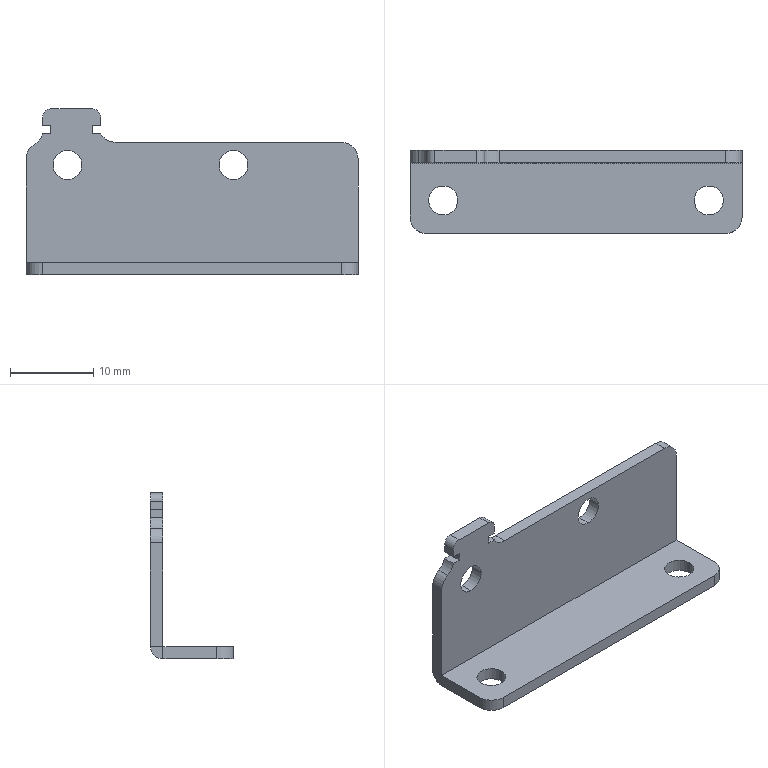Part | SolidWorks | features Fillet 3, ICE 3, FlatPattern 1, SMBaseFlange 1, SheetMetal 1 | 1 solid | 38 faces | box 40 x 10 x 20 mm | volume 1427 mm3 | plane 21 | cylinder 17 | commonest cylinder face diameters 3.5 x8 4 x6 2 x2 3 x1
STEP:
#1=CARTESIAN_POINT('',(5.75,-6.,-16.));
#2=VERTEX_POINT('',#1);
#3=CARTESIAN_POINT('',(2.25,-6.,-16.));
#4=VERTEX_POINT('',#3);
#5=CARTESIAN_POINT('',(4.,-6.,-16.));
#6=DIRECTION('',(0.,0.,-1.));
#7=DIRECTION('',(0.,1.,0.));
#8=AXIS2_PLACEMENT_3D('',#5,#6,#7);
#9=CIRCLE('',#8,1.75);
#10=EDGE_CURVE('',#2,#4,#9,.T.);
#11=ORIENTED_EDGE('',*,*,#10,.T.);
#12=CARTESIAN_POINT('',(2.25,-6.,-14.5));
#13=VERTEX_POINT('',#12);
#14=CARTESIAN_POINT('',(2.25,-6.,-24.5));
#15=DIRECTION('',(0.,0.,1.));
#16=VECTOR('',#15,1000.);
#17=LINE('',#14,#16);
#18=EDGE_CURVE('',#4,#13,#17,.T.);
#19=ORIENTED_EDGE('',*,*,#18,.T.);
#20=CARTESIAN_POINT('',(5.75,-6.,-14.5));
#21=VERTEX_POINT('',#20);
#22=CARTESIAN_POINT('',(4.,-6.,-14.5));
#23=DIRECTION('',(0.,0.,1.));
#24=DIRECTION('',(1.,0.,0.));
#25=AXIS2_PLACEMENT_3D('',#22,#23,#24);
#26=CIRCLE('',#25,1.75);
#27=EDGE_CURVE('',#13,#21,#26,.T.);
#28=ORIENTED_EDGE('',*,*,#27,.T.);
#29=CARTESIAN_POINT('',(5.75,-6.,-24.5));
#30=DIRECTION('',(0.,0.,1.));
#31=VECTOR('',#30,1000.);
#32=LINE('',#29,#31);
#33=EDGE_CURVE('',#2,#21,#32,.T.);
#34=ORIENTED_EDGE('',*,*,#33,.F.);
#35=EDGE_LOOP('',(#11,#19,#28,#34));
#36=FACE_OUTER_BOUND('',#35,.T.);
#37=CARTESIAN_POINT('',(4.,-6.,-24.5));
#38=DIRECTION('',(0.,0.,1.));
#39=DIRECTION('',(1.,0.,0.));
#40=AXIS2_PLACEMENT_3D('',#37,#38,#39);
#41=CYLINDRICAL_SURFACE('',#40,1.75);
#42=ADVANCED_FACE('',(#36),#41,.F.);
#43=CARTESIAN_POINT('',(37.75,-6.,-16.));
#44=VERTEX_POINT('',#43);
#45=CARTESIAN_POINT('',(34.25,-6.,-16.));
#46=VERTEX_POINT('',#45);
#47=CARTESIAN_POINT('',(36.,-6.,-16.));
#48=DIRECTION('',(0.,0.,-1.));
#49=DIRECTION('',(0.,1.,0.));
#50=AXIS2_PLACEMENT_3D('',#47,#48,#49);
#51=CIRCLE('',#50,1.75);
#52=EDGE_CURVE('',#44,#46,#51,.T.);
#53=ORIENTED_EDGE('',*,*,#52,.T.);
#54=CARTESIAN_POINT('',(34.25,-6.,-14.5));
#55=VERTEX_POINT('',#54);
#56=CARTESIAN_POINT('',(34.25,-6.,-24.5));
#57=DIRECTION('',(0.,0.,1.));
#58=VECTOR('',#57,1000.);
#59=LINE('',#56,#58);
#60=EDGE_CURVE('',#46,#55,#59,.T.);
#61=ORIENTED_EDGE('',*,*,#60,.T.);
#62=CARTESIAN_POINT('',(37.75,-6.,-14.5));
#63=VERTEX_POINT('',#62);
#64=CARTESIAN_POINT('',(36.,-6.,-14.5));
#65=DIRECTION('',(0.,0.,1.));
#66=DIRECTION('',(1.,0.,0.));
#67=AXIS2_PLACEMENT_3D('',#64,#65,#66);
#68=CIRCLE('',#67,1.75);
#69=EDGE_CURVE('',#55,#63,#68,.T.);
#70=ORIENTED_EDGE('',*,*,#69,.T.);
#71=CARTESIAN_POINT('',(37.75,-6.,-24.5));
#72=DIRECTION('',(0.,0.,1.));
#73=VECTOR('',#72,1000.);
#74=LINE('',#71,#73);
#75=EDGE_CURVE('',#44,#63,#74,.T.);
#76=ORIENTED_EDGE('',*,*,#75,.F.);
#77=EDGE_LOOP('',(#53,#61,#70,#76));
#78=FACE_OUTER_BOUND('',#77,.T.);
#79=CARTESIAN_POINT('',(36.,-6.,-24.5));
#80=DIRECTION('',(0.,0.,1.));
#81=DIRECTION('',(1.,0.,0.));
#82=AXIS2_PLACEMENT_3D('',#79,#80,#81);
#83=CYLINDRICAL_SURFACE('',#82,1.75);
#84=ADVANCED_FACE('',(#78),#83,.F.);
#85=CARTESIAN_POINT('',(5.,0.,-4.5));
#86=VERTEX_POINT('',#85);
#87=CARTESIAN_POINT('',(5.,0.,-1.));
#88=VERTEX_POINT('',#87);
#89=CARTESIAN_POINT('',(5.,0.,-2.75));
#90=DIRECTION('',(0.,1.,0.));
#91=DIRECTION('',(0.,0.,1.));
#92=AXIS2_PLACEMENT_3D('',#89,#90,#91);
#93=CIRCLE('',#92,1.75);
#94=EDGE_CURVE('',#86,#88,#93,.T.);
#95=ORIENTED_EDGE('',*,*,#94,.T.);
#96=CARTESIAN_POINT('',(5.,-1.5,-1.));
#97=VERTEX_POINT('',#96);
#98=CARTESIAN_POINT('',(5.,8.5,-1.));
#99=DIRECTION('',(0.,-1.,0.));
#100=VECTOR('',#99,1000.);
#101=LINE('',#98,#100);
#102=EDGE_CURVE('',#88,#97,#101,.T.);
#103=ORIENTED_EDGE('',*,*,#102,.T.);
#104=CARTESIAN_POINT('',(5.,-1.5,-4.5));
#105=VERTEX_POINT('',#104);
#106=CARTESIAN_POINT('',(5.,-1.5,-2.75));
#107=DIRECTION('',(0.,-1.,0.));
#108=DIRECTION('',(0.,0.,-1.));
#109=AXIS2_PLACEMENT_3D('',#106,#107,#108);
#110=CIRCLE('',#109,1.75);
#111=EDGE_CURVE('',#97,#105,#110,.T.);
#112=ORIENTED_EDGE('',*,*,#111,.T.);
#113=CARTESIAN_POINT('',(5.,8.5,-4.5));
#114=DIRECTION('',(0.,-1.,0.));
#115=VECTOR('',#114,1000.);
#116=LINE('',#113,#115);
#117=EDGE_CURVE('',#86,#105,#116,.T.);
#118=ORIENTED_EDGE('',*,*,#117,.F.);
#119=EDGE_LOOP('',(#95,#103,#112,#118));
#120=FACE_OUTER_BOUND('',#119,.T.);
#121=CARTESIAN_POINT('',(5.,8.5,-2.75));
#122=DIRECTION('',(0.,-1.,0.));
#123=DIRECTION('',(0.,0.,-1.));
#124=AXIS2_PLACEMENT_3D('',#121,#122,#123);
#125=CYLINDRICAL_SURFACE('',#124,1.75);
#126=ADVANCED_FACE('',(#120),#125,.F.);
#127=CARTESIAN_POINT('',(25.,0.,-4.5));
#128=VERTEX_POINT('',#127);
#129=CARTESIAN_POINT('',(25.,0.,-1.));
#130=VERTEX_POINT('',#129);
#131=CARTESIAN_POINT('',(25.,0.,-2.75));
#132=DIRECTION('',(0.,1.,0.));
#133=DIRECTION('',(0.,0.,1.));
#134=AXIS2_PLACEMENT_3D('',#131,#132,#133);
#135=CIRCLE('',#134,1.75);
#136=EDGE_CURVE('',#128,#130,#135,.T.);
#137=ORIENTED_EDGE('',*,*,#136,.T.);
#138=CARTESIAN_POINT('',(25.,-1.5,-1.));
#139=VERTEX_POINT('',#138);
#140=CARTESIAN_POINT('',(25.,8.5,-1.));
#141=DIRECTION('',(0.,-1.,0.));
#142=VECTOR('',#141,1000.);
#143=LINE('',#140,#142);
#144=EDGE_CURVE('',#130,#139,#143,.T.);
#145=ORIENTED_EDGE('',*,*,#144,.T.);
#146=CARTESIAN_POINT('',(25.,-1.5,-4.5));
#147=VERTEX_POINT('',#146);
#148=CARTESIAN_POINT('',(25.,-1.5,-2.75));
#149=DIRECTION('',(0.,-1.,0.));
#150=DIRECTION('',(0.,0.,-1.));
#151=AXIS2_PLACEMENT_3D('',#148,#149,#150);
#152=CIRCLE('',#151,1.75);
#153=EDGE_CURVE('',#139,#147,#152,.T.);
#154=ORIENTED_EDGE('',*,*,#153,.T.);
#155=CARTESIAN_POINT('',(25.,8.5,-4.5));
#156=DIRECTION('',(0.,-1.,0.));
#157=VECTOR('',#156,1000.);
#158=LINE('',#155,#157);
#159=EDGE_CURVE('',#128,#147,#158,.T.);
#160=ORIENTED_EDGE('',*,*,#159,.F.);
#161=EDGE_LOOP('',(#137,#145,#154,#160));
#162=FACE_OUTER_BOUND('',#161,.T.);
#163=CARTESIAN_POINT('',(25.,8.5,-2.75));
#164=DIRECTION('',(0.,-1.,0.));
#165=DIRECTION('',(0.,0.,-1.));
#166=AXIS2_PLACEMENT_3D('',#163,#164,#165);
#167=CYLINDRICAL_SURFACE('',#166,1.75);
#168=ADVANCED_FACE('',(#162),#167,.F.);
#169=CARTESIAN_POINT('',(40.,-1.5,-14.5));
#170=VERTEX_POINT('',#169);
#171=CARTESIAN_POINT('',(40.,-8.,-14.5));
#172=VERTEX_POINT('',#171);
#173=CARTESIAN_POINT('',(40.,0.,-14.5));
#174=DIRECTION('',(0.,-1.,0.));
#175=VECTOR('',#174,1000.);
#176=LINE('',#173,#175);
#177=EDGE_CURVE('',#170,#172,#176,.T.);
#178=ORIENTED_EDGE('',*,*,#177,.T.);
#179=CARTESIAN_POINT('',(40.,-8.,-16.));
#180=VERTEX_POINT('',#179);
#181=CARTESIAN_POINT('',(40.,-8.,-14.5));
#182=DIRECTION('',(0.,0.,-1.));
#183=VECTOR('',#182,1000.);
#184=LINE('',#181,#183);
#185=EDGE_CURVE('',#172,#180,#184,.T.);
#186=ORIENTED_EDGE('',*,*,#185,.T.);
#187=CARTESIAN_POINT('',(40.,-1.5,-16.));
#188=VERTEX_POINT('',#187);
#189=CARTESIAN_POINT('',(40.,0.,-16.));
#190=DIRECTION('',(0.,-1.,0.));
#191=VECTOR('',#190,1000.);
#192=LINE('',#189,#191);
#193=EDGE_CURVE('',#188,#180,#192,.T.);
#194=ORIENTED_EDGE('',*,*,#193,.F.);
#195=CARTESIAN_POINT('',(40.,-1.5,-14.5));
#196=DIRECTION('',(0.,0.,-1.));
#197=VECTOR('',#196,1000.);
#198=LINE('',#195,#197);
#199=EDGE_CURVE('',#170,#188,#198,.T.);
#200=ORIENTED_EDGE('',*,*,#199,.F.);
#201=EDGE_LOOP('',(#178,#186,#194,#200));
#202=FACE_OUTER_BOUND('',#201,.T.);
#203=CARTESIAN_POINT('',(40.,-1.5,-14.5));
#204=DIRECTION('',(1.,0.,0.));
#205=DIRECTION('',(0.,0.,-1.));
#206=AXIS2_PLACEMENT_3D('',#203,#204,#205);
#207=PLANE('',#206);
#208=ADVANCED_FACE('',(#202),#207,.T.);
#209=CARTESIAN_POINT('',(40.,0.,-14.5));
#210=VERTEX_POINT('',#209);
#211=CARTESIAN_POINT('',(40.,-1.5,-14.5));
#212=DIRECTION('',(0.,1.,0.));
#213=VECTOR('',#212,1000.);
#214=LINE('',#211,#213);
#215=EDGE_CURVE('',#170,#210,#214,.T.);
#216=ORIENTED_EDGE('',*,*,#215,.F.);
#217=ORIENTED_EDGE('',*,*,#199,.T.);
#218=CARTESIAN_POINT('',(40.,-1.5,-14.5));
#219=DIRECTION('',(-1.,0.,0.));
#220=DIRECTION('',(0.,0.,-1.));
#221=AXIS2_PLACEMENT_3D('',#218,#219,#220);
#222=CIRCLE('',#221,1.5);
#223=EDGE_CURVE('',#210,#188,#222,.T.);
#224=ORIENTED_EDGE('',*,*,#223,.F.);
#225=EDGE_LOOP('',(#216,#217,#224));
#226=FACE_OUTER_BOUND('',#225,.T.);
#227=CARTESIAN_POINT('',(40.,-1.5,-14.5));
#228=DIRECTION('',(1.,0.,0.));
#229=DIRECTION('',(0.,0.,-1.));
#230=AXIS2_PLACEMENT_3D('',#227,#228,#229);
#231=PLANE('',#230);
#232=ADVANCED_FACE('',(#226),#231,.T.);
#233=CARTESIAN_POINT('',(0.,-1.5,-2.));
#234=VERTEX_POINT('',#233);
#235=CARTESIAN_POINT('',(0.,-1.5,-14.5));
#236=VERTEX_POINT('',#235);
#237=CARTESIAN_POINT('',(0.,-1.5,0.));
#238=DIRECTION('',(0.,0.,-1.));
#239=VECTOR('',#238,1000.);
#240=LINE('',#237,#239);
#241=EDGE_CURVE('',#234,#236,#240,.T.);
#242=ORIENTED_EDGE('',*,*,#241,.F.);
#243=CARTESIAN_POINT('',(0.,0.,-2.));
#244=VERTEX_POINT('',#243);
#245=CARTESIAN_POINT('',(0.,-1.5,-2.));
#246=DIRECTION('',(0.,1.,0.));
#247=VECTOR('',#246,1000.);
#248=LINE('',#245,#247);
#249=EDGE_CURVE('',#234,#244,#248,.T.);
#250=ORIENTED_EDGE('',*,*,#249,.T.);
#251=CARTESIAN_POINT('',(0.,0.,-14.5));
#252=VERTEX_POINT('',#251);
#253=CARTESIAN_POINT('',(0.,0.,0.));
#254=DIRECTION('',(0.,0.,-1.));
#255=VECTOR('',#254,1000.);
#256=LINE('',#253,#255);
#257=EDGE_CURVE('',#244,#252,#256,.T.);
#258=ORIENTED_EDGE('',*,*,#257,.T.);
#259=CARTESIAN_POINT('',(0.,-1.5,-14.5));
#260=DIRECTION('',(0.,1.,0.));
#261=VECTOR('',#260,1000.);
#262=LINE('',#259,#261);
#263=EDGE_CURVE('',#236,#252,#262,.T.);
#264=ORIENTED_EDGE('',*,*,#263,.F.);
#265=EDGE_LOOP('',(#242,#250,#258,#264));
#266=FACE_OUTER_BOUND('',#265,.T.);
#267=CARTESIAN_POINT('',(0.,-1.5,-14.5));
#268=DIRECTION('',(-1.,0.,0.));
#269=DIRECTION('',(0.,0.,1.));
#270=AXIS2_PLACEMENT_3D('',#267,#268,#269);
#271=PLANE('',#270);
#272=ADVANCED_FACE('',(#266),#271,.T.);
#273=CARTESIAN_POINT('',(0.,-1.5,-16.));
#274=VERTEX_POINT('',#273);
#275=CARTESIAN_POINT('',(0.,-1.5,-14.5));
#276=DIRECTION('',(0.,0.,-1.));
#277=VECTOR('',#276,1000.);
#278=LINE('',#275,#277);
#279=EDGE_CURVE('',#236,#274,#278,.T.);
#280=ORIENTED_EDGE('',*,*,#279,.F.);
#281=ORIENTED_EDGE('',*,*,#263,.T.);
#282=CARTESIAN_POINT('',(0.,-1.5,-14.5));
#283=DIRECTION('',(-1.,0.,0.));
#284=DIRECTION('',(0.,0.,-1.));
#285=AXIS2_PLACEMENT_3D('',#282,#283,#284);
#286=CIRCLE('',#285,1.5);
#287=EDGE_CURVE('',#252,#274,#286,.T.);
#288=ORIENTED_EDGE('',*,*,#287,.T.);
#289=EDGE_LOOP('',(#280,#281,#288));
#290=FACE_OUTER_BOUND('',#289,.T.);
#291=CARTESIAN_POINT('',(0.,-1.5,-14.5));
#292=DIRECTION('',(-1.,0.,0.));
#293=DIRECTION('',(0.,0.,1.));
#294=AXIS2_PLACEMENT_3D('',#291,#292,#293);
#295=PLANE('',#294);
#296=ADVANCED_FACE('',(#290),#295,.T.);
#297=CARTESIAN_POINT('',(4.,-6.,-14.5));
#298=DIRECTION('',(0.,0.,1.));
#299=DIRECTION('',(1.,0.,0.));
#300=AXIS2_PLACEMENT_3D('',#297,#298,#299);
#301=CIRCLE('',#300,1.75);
#302=EDGE_CURVE('',#21,#13,#301,.T.);
#303=ORIENTED_EDGE('',*,*,#302,.F.);
#304=ORIENTED_EDGE('',*,*,#27,.F.);
#305=EDGE_LOOP('',(#303,#304));
#306=FACE_BOUND('',#305,.T.);
#307=CARTESIAN_POINT('',(36.,-6.,-14.5));
#308=DIRECTION('',(0.,0.,1.));
#309=DIRECTION('',(1.,0.,0.));
#310=AXIS2_PLACEMENT_3D('',#307,#308,#309);
#311=CIRCLE('',#310,1.75);
#312=EDGE_CURVE('',#63,#55,#311,.T.);
#313=ORIENTED_EDGE('',*,*,#312,.F.);
#314=ORIENTED_EDGE('',*,*,#69,.F.);
#315=EDGE_LOOP('',(#313,#314));
#316=FACE_BOUND('',#315,.T.);
#317=CARTESIAN_POINT('',(38.,-10.,-14.5));
#318=VERTEX_POINT('',#317);
#319=CARTESIAN_POINT('',(2.,-10.,-14.5));
#320=VERTEX_POINT('',#319);
#321=CARTESIAN_POINT('',(40.,-10.,-14.5));
#322=DIRECTION('',(-1.,0.,0.));
#323=VECTOR('',#322,1000.);
#324=LINE('',#321,#323);
#325=EDGE_CURVE('',#318,#320,#324,.T.);
#326=ORIENTED_EDGE('',*,*,#325,.F.);
#327=CARTESIAN_POINT('',(38.,-8.,-14.5));
#328=DIRECTION('',(0.,0.,1.));
#329=DIRECTION('',(0.,1.,0.));
#330=AXIS2_PLACEMENT_3D('',#327,#328,#329);
#331=CIRCLE('',#330,2.);
#332=EDGE_CURVE('',#318,#172,#331,.T.);
#333=ORIENTED_EDGE('',*,*,#332,.T.);
#334=ORIENTED_EDGE('',*,*,#177,.F.);
#335=CARTESIAN_POINT('',(40.,-1.5,-14.5));
#336=DIRECTION('',(-1.,0.,0.));
#337=VECTOR('',#336,1000.);
#338=LINE('',#335,#337);
#339=EDGE_CURVE('',#170,#236,#338,.T.);
#340=ORIENTED_EDGE('',*,*,#339,.T.);
#341=CARTESIAN_POINT('',(0.,-8.,-14.5));
#342=VERTEX_POINT('',#341);
#343=CARTESIAN_POINT('',(0.,0.,-14.5));
#344=DIRECTION('',(0.,-1.,0.));
#345=VECTOR('',#344,1000.);
#346=LINE('',#343,#345);
#347=EDGE_CURVE('',#236,#342,#346,.T.);
#348=ORIENTED_EDGE('',*,*,#347,.T.);
#349=CARTESIAN_POINT('',(2.,-8.,-14.5));
#350=DIRECTION('',(0.,0.,1.));
#351=DIRECTION('',(0.,1.,0.));
#352=AXIS2_PLACEMENT_3D('',#349,#350,#351);
#353=CIRCLE('',#352,2.);
#354=EDGE_CURVE('',#342,#320,#353,.T.);
#355=ORIENTED_EDGE('',*,*,#354,.T.);
#356=EDGE_LOOP('',(#326,#333,#334,#340,#348,#355));
#357=FACE_OUTER_BOUND('',#356,.T.);
#358=CARTESIAN_POINT('',(40.,0.,-14.5));
#359=DIRECTION('',(0.,0.,-1.));
#360=DIRECTION('',(0.,1.,0.));
#361=AXIS2_PLACEMENT_3D('',#358,#359,#360);
#362=PLANE('',#361);
#363=ADVANCED_FACE('',(#306,#316,#357),#362,.F.);
#364=CARTESIAN_POINT('',(38.,-10.,-16.));
#365=VERTEX_POINT('',#364);
#366=CARTESIAN_POINT('',(2.,-10.,-16.));
#367=VERTEX_POINT('',#366);
#368=CARTESIAN_POINT('',(40.,-10.,-16.));
#369=DIRECTION('',(-1.,0.,0.));
#370=VECTOR('',#369,1000.);
#371=LINE('',#368,#370);
#372=EDGE_CURVE('',#365,#367,#371,.T.);
#373=ORIENTED_EDGE('',*,*,#372,.F.);
#374=CARTESIAN_POINT('',(38.,-10.,-16.));
#375=DIRECTION('',(0.,0.,1.));
#376=VECTOR('',#375,1000.);
#377=LINE('',#374,#376);
#378=EDGE_CURVE('',#365,#318,#377,.T.);
#379=ORIENTED_EDGE('',*,*,#378,.T.);
#380=ORIENTED_EDGE('',*,*,#325,.T.);
#381=CARTESIAN_POINT('',(2.,-10.,-16.));
#382=DIRECTION('',(0.,0.,-1.));
#383=VECTOR('',#382,1000.);
#384=LINE('',#381,#383);
#385=EDGE_CURVE('',#320,#367,#384,.T.);
#386=ORIENTED_EDGE('',*,*,#385,.T.);
#387=EDGE_LOOP('',(#373,#379,#380,#386));
#388=FACE_OUTER_BOUND('',#387,.T.);
#389=CARTESIAN_POINT('',(40.,-10.,-16.));
#390=DIRECTION('',(0.,-1.,0.));
#391=DIRECTION('',(0.,0.,-1.));
#392=AXIS2_PLACEMENT_3D('',#389,#390,#391);
#393=PLANE('',#392);
#394=ADVANCED_FACE('',(#388),#393,.T.);
#395=ORIENTED_EDGE('',*,*,#10,.F.);
#396=CARTESIAN_POINT('',(4.,-6.,-16.));
#397=DIRECTION('',(0.,0.,-1.));
#398=DIRECTION('',(0.,1.,0.));
#399=AXIS2_PLACEMENT_3D('',#396,#397,#398);
#400=CIRCLE('',#399,1.75);
#401=EDGE_CURVE('',#4,#2,#400,.T.);
#402=ORIENTED_EDGE('',*,*,#401,.F.);
#403=EDGE_LOOP('',(#395,#402));
#404=FACE_BOUND('',#403,.T.);
#405=ORIENTED_EDGE('',*,*,#52,.F.);
#406=CARTESIAN_POINT('',(36.,-6.,-16.));
#407=DIRECTION('',(0.,0.,-1.));
#408=DIRECTION('',(0.,1.,0.));
#409=AXIS2_PLACEMENT_3D('',#406,#407,#408);
#410=CIRCLE('',#409,1.75);
#411=EDGE_CURVE('',#46,#44,#410,.T.);
#412=ORIENTED_EDGE('',*,*,#411,.F.);
#413=EDGE_LOOP('',(#405,#412));
#414=FACE_BOUND('',#413,.T.);
#415=ORIENTED_EDGE('',*,*,#193,.T.);
#416=CARTESIAN_POINT('',(38.,-8.,-16.));
#417=DIRECTION('',(0.,0.,-1.));
#418=DIRECTION('',(0.,1.,0.));
#419=AXIS2_PLACEMENT_3D('',#416,#417,#418);
#420=CIRCLE('',#419,2.);
#421=EDGE_CURVE('',#180,#365,#420,.T.);
#422=ORIENTED_EDGE('',*,*,#421,.T.);
#423=ORIENTED_EDGE('',*,*,#372,.T.);
#424=CARTESIAN_POINT('',(0.,-8.,-16.));
#425=VERTEX_POINT('',#424);
#426=CARTESIAN_POINT('',(2.,-8.,-16.));
#427=DIRECTION('',(0.,0.,-1.));
#428=DIRECTION('',(0.,1.,0.));
#429=AXIS2_PLACEMENT_3D('',#426,#427,#428);
#430=CIRCLE('',#429,2.);
#431=EDGE_CURVE('',#367,#425,#430,.T.);
#432=ORIENTED_EDGE('',*,*,#431,.T.);
#433=CARTESIAN_POINT('',(0.,0.,-16.));
#434=DIRECTION('',(0.,-1.,0.));
#435=VECTOR('',#434,1000.);
#436=LINE('',#433,#435);
#437=EDGE_CURVE('',#274,#425,#436,.T.);
#438=ORIENTED_EDGE('',*,*,#437,.F.);
#439=CARTESIAN_POINT('',(40.,-1.5,-16.));
#440=DIRECTION('',(-1.,0.,0.));
#441=VECTOR('',#440,1000.);
#442=LINE('',#439,#441);
#443=EDGE_CURVE('',#188,#274,#442,.T.);
#444=ORIENTED_EDGE('',*,*,#443,.F.);
#445=EDGE_LOOP('',(#415,#422,#423,#432,#438,#444));
#446=FACE_OUTER_BOUND('',#445,.T.);
#447=CARTESIAN_POINT('',(40.,0.,-16.));
#448=DIRECTION('',(0.,0.,-1.));
#449=DIRECTION('',(0.,1.,0.));
#450=AXIS2_PLACEMENT_3D('',#447,#448,#449);
#451=PLANE('',#450);
#452=ADVANCED_FACE('',(#404,#414,#446),#451,.T.);
#453=ORIENTED_EDGE('',*,*,#287,.F.);
#454=CARTESIAN_POINT('',(40.,0.,-14.5));
#455=DIRECTION('',(-1.,0.,0.));
#456=VECTOR('',#455,1000.);
#457=LINE('',#454,#456);
#458=EDGE_CURVE('',#210,#252,#457,.T.);
#459=ORIENTED_EDGE('',*,*,#458,.F.);
#460=ORIENTED_EDGE('',*,*,#223,.T.);
#461=ORIENTED_EDGE('',*,*,#443,.T.);
#462=EDGE_LOOP('',(#453,#459,#460,#461));
#463=FACE_OUTER_BOUND('',#462,.T.);
#464=CARTESIAN_POINT('',(40.,-1.5,-14.5));
#465=DIRECTION('',(-1.,0.,0.));
#466=DIRECTION('',(0.,0.,1.));
#467=AXIS2_PLACEMENT_3D('',#464,#465,#466);
#468=CYLINDRICAL_SURFACE('',#467,1.5);
#469=ADVANCED_FACE('',(#463),#468,.T.);
#470=ORIENTED_EDGE('',*,*,#94,.F.);
#471=CARTESIAN_POINT('',(5.,0.,-2.75));
#472=DIRECTION('',(0.,1.,0.));
#473=DIRECTION('',(0.,0.,1.));
#474=AXIS2_PLACEMENT_3D('',#471,#472,#473);
#475=CIRCLE('',#474,1.75);
#476=EDGE_CURVE('',#88,#86,#475,.T.);
#477=ORIENTED_EDGE('',*,*,#476,.F.);
#478=EDGE_LOOP('',(#470,#477));
#479=FACE_BOUND('',#478,.T.);
#480=ORIENTED_EDGE('',*,*,#136,.F.);
#481=CARTESIAN_POINT('',(25.,0.,-2.75));
#482=DIRECTION('',(0.,1.,0.));
#483=DIRECTION('',(0.,0.,1.));
#484=AXIS2_PLACEMENT_3D('',#481,#482,#483);
#485=CIRCLE('',#484,1.75);
#486=EDGE_CURVE('',#130,#128,#485,.T.);
#487=ORIENTED_EDGE('',*,*,#486,.F.);
#488=EDGE_LOOP('',(#480,#487));
#489=FACE_BOUND('',#488,.T.);
#490=CARTESIAN_POINT('',(2.,0.,2.));
#491=VERTEX_POINT('',#490);
#492=CARTESIAN_POINT('',(2.,0.,3.));
#493=VERTEX_POINT('',#492);
#494=CARTESIAN_POINT('',(2.,0.,4.));
#495=DIRECTION('',(0.,0.,1.));
#496=VECTOR('',#495,1000.);
#497=LINE('',#494,#496);
#498=EDGE_CURVE('',#491,#493,#497,.T.);
#499=ORIENTED_EDGE('',*,*,#498,.T.);
#500=CARTESIAN_POINT('',(3.,0.,4.));
#501=VERTEX_POINT('',#500);
#502=CARTESIAN_POINT('',(3.,0.,3.));
#503=DIRECTION('',(0.,1.,0.));
#504=DIRECTION('',(0.,0.,1.));
#505=AXIS2_PLACEMENT_3D('',#502,#503,#504);
#506=CIRCLE('',#505,1.);
#507=EDGE_CURVE('',#493,#501,#506,.T.);
#508=ORIENTED_EDGE('',*,*,#507,.T.);
#509=CARTESIAN_POINT('',(8.,0.,4.));
#510=VERTEX_POINT('',#509);
#511=CARTESIAN_POINT('',(9.,0.,4.));
#512=DIRECTION('',(1.,0.,0.));
#513=VECTOR('',#512,1000.);
#514=LINE('',#511,#513);
#515=EDGE_CURVE('',#501,#510,#514,.T.);
#516=ORIENTED_EDGE('',*,*,#515,.T.);
#517=CARTESIAN_POINT('',(9.,0.,3.));
#518=VERTEX_POINT('',#517);
#519=CARTESIAN_POINT('',(8.,0.,3.));
#520=DIRECTION('',(0.,1.,0.));
#521=DIRECTION('',(0.,0.,1.));
#522=AXIS2_PLACEMENT_3D('',#519,#520,#521);
#523=CIRCLE('',#522,1.);
#524=EDGE_CURVE('',#510,#518,#523,.T.);
#525=ORIENTED_EDGE('',*,*,#524,.T.);
#526=CARTESIAN_POINT('',(9.,0.,2.));
#527=VERTEX_POINT('',#526);
#528=CARTESIAN_POINT('',(9.,0.,2.));
#529=DIRECTION('',(0.,0.,-1.));
#530=VECTOR('',#529,1000.);
#531=LINE('',#528,#530);
#532=EDGE_CURVE('',#518,#527,#531,.T.);
#533=ORIENTED_EDGE('',*,*,#532,.T.);
#534=CARTESIAN_POINT('',(8.,0.,2.));
#535=VERTEX_POINT('',#534);
#536=CARTESIAN_POINT('',(8.,0.,2.));
#537=DIRECTION('',(-1.,0.,0.));
#538=VECTOR('',#537,1000.);
#539=LINE('',#536,#538);
#540=EDGE_CURVE('',#527,#535,#539,.T.);
#541=ORIENTED_EDGE('',*,*,#540,.T.);
#542=CARTESIAN_POINT('',(8.,0.,1.));
#543=VERTEX_POINT('',#542);
#544=CARTESIAN_POINT('',(8.,0.,1.));
#545=DIRECTION('',(0.,0.,-1.));
#546=VECTOR('',#545,1000.);
#547=LINE('',#544,#546);
#548=EDGE_CURVE('',#535,#543,#547,.T.);
#549=ORIENTED_EDGE('',*,*,#548,.T.);
#550=CARTESIAN_POINT('',(9.,0.,1.));
#551=VERTEX_POINT('',#550);
#552=CARTESIAN_POINT('',(8.,0.,1.));
#553=DIRECTION('',(1.,0.,0.));
#554=VECTOR('',#553,1000.);
#555=LINE('',#552,#554);
#556=EDGE_CURVE('',#543,#551,#555,.T.);
#557=ORIENTED_EDGE('',*,*,#556,.T.);
#558=CARTESIAN_POINT('',(10.732,0.,0.));
#559=VERTEX_POINT('',#558);
#560=CARTESIAN_POINT('',(10.732,0.,2.));
#561=DIRECTION('',(0.,-1.,0.));
#562=DIRECTION('',(0.,0.,1.));
#563=AXIS2_PLACEMENT_3D('',#560,#561,#562);
#564=CIRCLE('',#563,2.);
#565=EDGE_CURVE('',#551,#559,#564,.T.);
#566=ORIENTED_EDGE('',*,*,#565,.T.);
#567=CARTESIAN_POINT('',(38.,0.,0.));
#568=VERTEX_POINT('',#567);
#569=CARTESIAN_POINT('',(40.,0.,0.));
#570=DIRECTION('',(-1.,0.,0.));
#571=VECTOR('',#570,1000.);
#572=LINE('',#569,#571);
#573=EDGE_CURVE('',#568,#559,#572,.T.);
#574=ORIENTED_EDGE('',*,*,#573,.F.);
#575=CARTESIAN_POINT('',(40.,0.,-2.));
#576=VERTEX_POINT('',#575);
#577=CARTESIAN_POINT('',(38.,0.,-2.));
#578=DIRECTION('',(0.,1.,0.));
#579=DIRECTION('',(0.,0.,1.));
#580=AXIS2_PLACEMENT_3D('',#577,#578,#579);
#581=CIRCLE('',#580,2.);
#582=EDGE_CURVE('',#568,#576,#581,.T.);
#583=ORIENTED_EDGE('',*,*,#582,.T.);
#584=CARTESIAN_POINT('',(40.,0.,0.));
#585=DIRECTION('',(0.,0.,-1.));
#586=VECTOR('',#585,1000.);
#587=LINE('',#584,#586);
#588=EDGE_CURVE('',#576,#210,#587,.T.);
#589=ORIENTED_EDGE('',*,*,#588,.T.);
#590=ORIENTED_EDGE('',*,*,#458,.T.);
#591=ORIENTED_EDGE('',*,*,#257,.F.);
#592=CARTESIAN_POINT('',(1.032,0.,-0.25));
#593=VERTEX_POINT('',#592);
#594=CARTESIAN_POINT('',(2.,0.,-2.));
#595=DIRECTION('',(0.,1.,0.));
#596=DIRECTION('',(0.,0.,1.));
#597=AXIS2_PLACEMENT_3D('',#594,#595,#596);
#598=CIRCLE('',#597,2.);
#599=EDGE_CURVE('',#244,#593,#598,.T.);
#600=ORIENTED_EDGE('',*,*,#599,.T.);
#601=CARTESIAN_POINT('',(2.,0.,1.));
#602=VERTEX_POINT('',#601);
#603=CARTESIAN_POINT('',(0.06351,0.,1.5));
#604=DIRECTION('',(0.,-1.,0.));
#605=DIRECTION('',(0.,0.,1.));
#606=AXIS2_PLACEMENT_3D('',#603,#604,#605);
#607=CIRCLE('',#606,2.);
#608=EDGE_CURVE('',#593,#602,#607,.T.);
#609=ORIENTED_EDGE('',*,*,#608,.T.);
#610=CARTESIAN_POINT('',(3.,0.,1.));
#611=VERTEX_POINT('',#610);
#612=CARTESIAN_POINT('',(3.,0.,1.));
#613=DIRECTION('',(1.,0.,0.));
#614=VECTOR('',#613,1000.);
#615=LINE('',#612,#614);
#616=EDGE_CURVE('',#602,#611,#615,.T.);
#617=ORIENTED_EDGE('',*,*,#616,.T.);
#618=CARTESIAN_POINT('',(3.,0.,2.));
#619=VERTEX_POINT('',#618);
#620=CARTESIAN_POINT('',(3.,0.,2.));
#621=DIRECTION('',(0.,0.,1.));
#622=VECTOR('',#621,1000.);
#623=LINE('',#620,#622);
#624=EDGE_CURVE('',#611,#619,#623,.T.);
#625=ORIENTED_EDGE('',*,*,#624,.T.);
#626=CARTESIAN_POINT('',(2.,0.,2.));
#627=DIRECTION('',(-1.,0.,0.));
#628=VECTOR('',#627,1000.);
#629=LINE('',#626,#628);
#630=EDGE_CURVE('',#619,#491,#629,.T.);
#631=ORIENTED_EDGE('',*,*,#630,.T.);
#632=EDGE_LOOP('',(#499,#508,#516,#525,#533,#541,#549,#557,#566,#574,#583,#589,#590,#591,#600,#609,#617,#625,#631));
#633=FACE_OUTER_BOUND('',#632,.T.);
#634=CARTESIAN_POINT('',(40.,0.,0.));
#635=DIRECTION('',(0.,1.,0.));
#636=DIRECTION('',(0.,0.,1.));
#637=AXIS2_PLACEMENT_3D('',#634,#635,#636);
#638=PLANE('',#637);
#639=ADVANCED_FACE('',(#479,#489,#633),#638,.T.);
#640=ORIENTED_EDGE('',*,*,#573,.T.);
#641=CARTESIAN_POINT('',(10.732,-1.5,0.));
#642=VERTEX_POINT('',#641);
#643=CARTESIAN_POINT('',(10.732,-1.5,0.));
#644=DIRECTION('',(0.,-1.,0.));
#645=VECTOR('',#644,1000.);
#646=LINE('',#643,#645);
#647=EDGE_CURVE('',#559,#642,#646,.T.);
#648=ORIENTED_EDGE('',*,*,#647,.T.);
#649=CARTESIAN_POINT('',(38.,-1.5,0.));
#650=VERTEX_POINT('',#649);
#651=CARTESIAN_POINT('',(40.,-1.5,0.));
#652=DIRECTION('',(-1.,0.,0.));
#653=VECTOR('',#652,1000.);
#654=LINE('',#651,#653);
#655=EDGE_CURVE('',#650,#642,#654,.T.);
#656=ORIENTED_EDGE('',*,*,#655,.F.);
#657=CARTESIAN_POINT('',(38.,-1.5,0.));
#658=DIRECTION('',(0.,1.,0.));
#659=VECTOR('',#658,1000.);
#660=LINE('',#657,#659);
#661=EDGE_CURVE('',#650,#568,#660,.T.);
#662=ORIENTED_EDGE('',*,*,#661,.T.);
#663=EDGE_LOOP('',(#640,#648,#656,#662));
#664=FACE_OUTER_BOUND('',#663,.T.);
#665=CARTESIAN_POINT('',(40.,-1.5,0.));
#666=DIRECTION('',(0.,0.,1.));
#667=DIRECTION('',(1.,0.,0.));
#668=AXIS2_PLACEMENT_3D('',#665,#666,#667);
#669=PLANE('',#668);
#670=ADVANCED_FACE('',(#664),#669,.T.);
#671=CARTESIAN_POINT('',(5.,-1.5,-2.75));
#672=DIRECTION('',(0.,-1.,0.));
#673=DIRECTION('',(0.,0.,-1.));
#674=AXIS2_PLACEMENT_3D('',#671,#672,#673);
#675=CIRCLE('',#674,1.75);
#676=EDGE_CURVE('',#105,#97,#675,.T.);
#677=ORIENTED_EDGE('',*,*,#676,.F.);
#678=ORIENTED_EDGE('',*,*,#111,.F.);
#679=EDGE_LOOP('',(#677,#678));
#680=FACE_BOUND('',#679,.T.);
#681=CARTESIAN_POINT('',(25.,-1.5,-2.75));
#682=DIRECTION('',(0.,-1.,0.));
#683=DIRECTION('',(0.,0.,-1.));
#684=AXIS2_PLACEMENT_3D('',#681,#682,#683);
#685=CIRCLE('',#684,1.75);
#686=EDGE_CURVE('',#147,#139,#685,.T.);
#687=ORIENTED_EDGE('',*,*,#686,.F.);
#688=ORIENTED_EDGE('',*,*,#153,.F.);
#689=EDGE_LOOP('',(#687,#688));
#690=FACE_BOUND('',#689,.T.);
#691=CARTESIAN_POINT('',(3.,-1.5,4.));
#692=VERTEX_POINT('',#691);
#693=CARTESIAN_POINT('',(8.,-1.5,4.));
#694=VERTEX_POINT('',#693);
#695=CARTESIAN_POINT('',(9.,-1.5,4.));
#696=DIRECTION('',(1.,0.,0.));
#697=VECTOR('',#696,1000.);
#698=LINE('',#695,#697);
#699=EDGE_CURVE('',#692,#694,#698,.T.);
#700=ORIENTED_EDGE('',*,*,#699,.F.);
#701=CARTESIAN_POINT('',(2.,-1.5,3.));
#702=VERTEX_POINT('',#701);
#703=CARTESIAN_POINT('',(3.,-1.5,3.));
#704=DIRECTION('',(0.,-1.,0.));
#705=DIRECTION('',(0.,0.,1.));
#706=AXIS2_PLACEMENT_3D('',#703,#704,#705);
#707=CIRCLE('',#706,1.);
#708=EDGE_CURVE('',#692,#702,#707,.T.);
#709=ORIENTED_EDGE('',*,*,#708,.T.);
#710=CARTESIAN_POINT('',(2.,-1.5,2.));
#711=VERTEX_POINT('',#710);
#712=CARTESIAN_POINT('',(2.,-1.5,4.));
#713=DIRECTION('',(0.,0.,1.));
#714=VECTOR('',#713,1000.);
#715=LINE('',#712,#714);
#716=EDGE_CURVE('',#711,#702,#715,.T.);
#717=ORIENTED_EDGE('',*,*,#716,.F.);
#718=CARTESIAN_POINT('',(3.,-1.5,2.));
#719=VERTEX_POINT('',#718);
#720=CARTESIAN_POINT('',(2.,-1.5,2.));
#721=DIRECTION('',(-1.,0.,0.));
#722=VECTOR('',#721,1000.);
#723=LINE('',#720,#722);
#724=EDGE_CURVE('',#719,#711,#723,.T.);
#725=ORIENTED_EDGE('',*,*,#724,.F.);
#726=CARTESIAN_POINT('',(3.,-1.5,1.));
#727=VERTEX_POINT('',#726);
#728=CARTESIAN_POINT('',(3.,-1.5,2.));
#729=DIRECTION('',(0.,0.,1.));
#730=VECTOR('',#729,1000.);
#731=LINE('',#728,#730);
#732=EDGE_CURVE('',#727,#719,#731,.T.);
#733=ORIENTED_EDGE('',*,*,#732,.F.);
#734=CARTESIAN_POINT('',(2.,-1.5,1.));
#735=VERTEX_POINT('',#734);
#736=CARTESIAN_POINT('',(3.,-1.5,1.));
#737=DIRECTION('',(1.,0.,0.));
#738=VECTOR('',#737,1000.);
#739=LINE('',#736,#738);
#740=EDGE_CURVE('',#735,#727,#739,.T.);
#741=ORIENTED_EDGE('',*,*,#740,.F.);
#742=CARTESIAN_POINT('',(1.032,-1.5,-0.25));
#743=VERTEX_POINT('',#742);
#744=CARTESIAN_POINT('',(0.06351,-1.5,1.5));
#745=DIRECTION('',(0.,1.,0.));
#746=DIRECTION('',(0.,0.,1.));
#747=AXIS2_PLACEMENT_3D('',#744,#745,#746);
#748=CIRCLE('',#747,2.);
#749=EDGE_CURVE('',#735,#743,#748,.T.);
#750=ORIENTED_EDGE('',*,*,#749,.T.);
#751=CARTESIAN_POINT('',(2.,-1.5,-2.));
#752=DIRECTION('',(0.,-1.,0.));
#753=DIRECTION('',(0.,0.,1.));
#754=AXIS2_PLACEMENT_3D('',#751,#752,#753);
#755=CIRCLE('',#754,2.);
#756=EDGE_CURVE('',#743,#234,#755,.T.);
#757=ORIENTED_EDGE('',*,*,#756,.T.);
#758=ORIENTED_EDGE('',*,*,#241,.T.);
#759=ORIENTED_EDGE('',*,*,#339,.F.);
#760=CARTESIAN_POINT('',(40.,-1.5,-2.));
#761=VERTEX_POINT('',#760);
#762=CARTESIAN_POINT('',(40.,-1.5,0.));
#763=DIRECTION('',(0.,0.,-1.));
#764=VECTOR('',#763,1000.);
#765=LINE('',#762,#764);
#766=EDGE_CURVE('',#761,#170,#765,.T.);
#767=ORIENTED_EDGE('',*,*,#766,.F.);
#768=CARTESIAN_POINT('',(38.,-1.5,-2.));
#769=DIRECTION('',(0.,-1.,0.));
#770=DIRECTION('',(0.,0.,1.));
#771=AXIS2_PLACEMENT_3D('',#768,#769,#770);
#772=CIRCLE('',#771,2.);
#773=EDGE_CURVE('',#761,#650,#772,.T.);
#774=ORIENTED_EDGE('',*,*,#773,.T.);
#775=ORIENTED_EDGE('',*,*,#655,.T.);
#776=CARTESIAN_POINT('',(9.,-1.5,1.));
#777=VERTEX_POINT('',#776);
#778=CARTESIAN_POINT('',(10.732,-1.5,2.));
#779=DIRECTION('',(0.,1.,0.));
#780=DIRECTION('',(0.,0.,1.));
#781=AXIS2_PLACEMENT_3D('',#778,#779,#780);
#782=CIRCLE('',#781,2.);
#783=EDGE_CURVE('',#642,#777,#782,.T.);
#784=ORIENTED_EDGE('',*,*,#783,.T.);
#785=CARTESIAN_POINT('',(8.,-1.5,1.));
#786=VERTEX_POINT('',#785);
#787=CARTESIAN_POINT('',(8.,-1.5,1.));
#788=DIRECTION('',(1.,0.,0.));
#789=VECTOR('',#788,1000.);
#790=LINE('',#787,#789);
#791=EDGE_CURVE('',#786,#777,#790,.T.);
#792=ORIENTED_EDGE('',*,*,#791,.F.);
#793=CARTESIAN_POINT('',(8.,-1.5,2.));
#794=VERTEX_POINT('',#793);
#795=CARTESIAN_POINT('',(8.,-1.5,1.));
#796=DIRECTION('',(0.,0.,-1.));
#797=VECTOR('',#796,1000.);
#798=LINE('',#795,#797);
#799=EDGE_CURVE('',#794,#786,#798,.T.);
#800=ORIENTED_EDGE('',*,*,#799,.F.);
#801=CARTESIAN_POINT('',(9.,-1.5,2.));
#802=VERTEX_POINT('',#801);
#803=CARTESIAN_POINT('',(8.,-1.5,2.));
#804=DIRECTION('',(-1.,0.,0.));
#805=VECTOR('',#804,1000.);
#806=LINE('',#803,#805);
#807=EDGE_CURVE('',#802,#794,#806,.T.);
#808=ORIENTED_EDGE('',*,*,#807,.F.);
#809=CARTESIAN_POINT('',(9.,-1.5,3.));
#810=VERTEX_POINT('',#809);
#811=CARTESIAN_POINT('',(9.,-1.5,2.));
#812=DIRECTION('',(0.,0.,-1.));
#813=VECTOR('',#812,1000.);
#814=LINE('',#811,#813);
#815=EDGE_CURVE('',#810,#802,#814,.T.);
#816=ORIENTED_EDGE('',*,*,#815,.F.);
#817=CARTESIAN_POINT('',(8.,-1.5,3.));
#818=DIRECTION('',(0.,-1.,0.));
#819=DIRECTION('',(0.,0.,1.));
#820=AXIS2_PLACEMENT_3D('',#817,#818,#819);
#821=CIRCLE('',#820,1.);
#822=EDGE_CURVE('',#810,#694,#821,.T.);
#823=ORIENTED_EDGE('',*,*,#822,.T.);
#824=EDGE_LOOP('',(#700,#709,#717,#725,#733,#741,#750,#757,#758,#759,#767,#774,#775,#784,#792,#800,#808,#816,#823));
#825=FACE_OUTER_BOUND('',#824,.T.);
#826=CARTESIAN_POINT('',(40.,-1.5,0.));
#827=DIRECTION('',(0.,1.,0.));
#828=DIRECTION('',(0.,0.,1.));
#829=AXIS2_PLACEMENT_3D('',#826,#827,#828);
#830=PLANE('',#829);
#831=ADVANCED_FACE('',(#680,#690,#825),#830,.F.);
#832=ORIENTED_EDGE('',*,*,#588,.F.);
#833=CARTESIAN_POINT('',(40.,-1.5,-2.));
#834=DIRECTION('',(0.,-1.,0.));
#835=VECTOR('',#834,1000.);
#836=LINE('',#833,#835);
#837=EDGE_CURVE('',#576,#761,#836,.T.);
#838=ORIENTED_EDGE('',*,*,#837,.T.);
#839=ORIENTED_EDGE('',*,*,#766,.T.);
#840=ORIENTED_EDGE('',*,*,#215,.T.);
#841=EDGE_LOOP('',(#832,#838,#839,#840));
#842=FACE_OUTER_BOUND('',#841,.T.);
#843=CARTESIAN_POINT('',(40.,-1.5,-14.5));
#844=DIRECTION('',(1.,0.,0.));
#845=DIRECTION('',(0.,0.,-1.));
#846=AXIS2_PLACEMENT_3D('',#843,#844,#845);
#847=PLANE('',#846);
#848=ADVANCED_FACE('',(#842),#847,.T.);
#849=ORIENTED_EDGE('',*,*,#437,.T.);
#850=CARTESIAN_POINT('',(0.,-8.,-14.5));
#851=DIRECTION('',(0.,0.,1.));
#852=VECTOR('',#851,1000.);
#853=LINE('',#850,#852);
#854=EDGE_CURVE('',#425,#342,#853,.T.);
#855=ORIENTED_EDGE('',*,*,#854,.T.);
#856=ORIENTED_EDGE('',*,*,#347,.F.);
#857=ORIENTED_EDGE('',*,*,#279,.T.);
#858=EDGE_LOOP('',(#849,#855,#856,#857));
#859=FACE_OUTER_BOUND('',#858,.T.);
#860=CARTESIAN_POINT('',(0.,-1.5,-14.5));
#861=DIRECTION('',(1.,0.,0.));
#862=DIRECTION('',(0.,0.,-1.));
#863=AXIS2_PLACEMENT_3D('',#860,#861,#862);
#864=PLANE('',#863);
#865=ADVANCED_FACE('',(#859),#864,.F.);
#866=ORIENTED_EDGE('',*,*,#144,.F.);
#867=ORIENTED_EDGE('',*,*,#486,.T.);
#868=ORIENTED_EDGE('',*,*,#159,.T.);
#869=ORIENTED_EDGE('',*,*,#686,.T.);
#870=EDGE_LOOP('',(#866,#867,#868,#869));
#871=FACE_OUTER_BOUND('',#870,.T.);
#872=CARTESIAN_POINT('',(25.,8.5,-2.75));
#873=DIRECTION('',(0.,-1.,0.));
#874=DIRECTION('',(0.,0.,-1.));
#875=AXIS2_PLACEMENT_3D('',#872,#873,#874);
#876=CYLINDRICAL_SURFACE('',#875,1.75);
#877=ADVANCED_FACE('',(#871),#876,.F.);
#878=ORIENTED_EDGE('',*,*,#102,.F.);
#879=ORIENTED_EDGE('',*,*,#476,.T.);
#880=ORIENTED_EDGE('',*,*,#117,.T.);
#881=ORIENTED_EDGE('',*,*,#676,.T.);
#882=EDGE_LOOP('',(#878,#879,#880,#881));
#883=FACE_OUTER_BOUND('',#882,.T.);
#884=CARTESIAN_POINT('',(5.,8.5,-2.75));
#885=DIRECTION('',(0.,-1.,0.));
#886=DIRECTION('',(0.,0.,-1.));
#887=AXIS2_PLACEMENT_3D('',#884,#885,#886);
#888=CYLINDRICAL_SURFACE('',#887,1.75);
#889=ADVANCED_FACE('',(#883),#888,.F.);
#890=ORIENTED_EDGE('',*,*,#60,.F.);
#891=ORIENTED_EDGE('',*,*,#411,.T.);
#892=ORIENTED_EDGE('',*,*,#75,.T.);
#893=ORIENTED_EDGE('',*,*,#312,.T.);
#894=EDGE_LOOP('',(#890,#891,#892,#893));
#895=FACE_OUTER_BOUND('',#894,.T.);
#896=CARTESIAN_POINT('',(36.,-6.,-24.5));
#897=DIRECTION('',(0.,0.,1.));
#898=DIRECTION('',(1.,0.,0.));
#899=AXIS2_PLACEMENT_3D('',#896,#897,#898);
#900=CYLINDRICAL_SURFACE('',#899,1.75);
#901=ADVANCED_FACE('',(#895),#900,.F.);
#902=ORIENTED_EDGE('',*,*,#18,.F.);
#903=ORIENTED_EDGE('',*,*,#401,.T.);
#904=ORIENTED_EDGE('',*,*,#33,.T.);
#905=ORIENTED_EDGE('',*,*,#302,.T.);
#906=EDGE_LOOP('',(#902,#903,#904,#905));
#907=FACE_OUTER_BOUND('',#906,.T.);
#908=CARTESIAN_POINT('',(4.,-6.,-24.5));
#909=DIRECTION('',(0.,0.,1.));
#910=DIRECTION('',(1.,0.,0.));
#911=AXIS2_PLACEMENT_3D('',#908,#909,#910);
#912=CYLINDRICAL_SURFACE('',#911,1.75);
#913=ADVANCED_FACE('',(#907),#912,.F.);
#914=ORIENTED_EDGE('',*,*,#556,.F.);
#915=CARTESIAN_POINT('',(8.,-1.5,1.));
#916=DIRECTION('',(0.,1.,0.));
#917=VECTOR('',#916,1000.);
#918=LINE('',#915,#917);
#919=EDGE_CURVE('',#786,#543,#918,.T.);
#920=ORIENTED_EDGE('',*,*,#919,.F.);
#921=ORIENTED_EDGE('',*,*,#791,.T.);
#922=CARTESIAN_POINT('',(9.,-1.5,1.));
#923=DIRECTION('',(0.,1.,0.));
#924=VECTOR('',#923,1000.);
#925=LINE('',#922,#924);
#926=EDGE_CURVE('',#777,#551,#925,.T.);
#927=ORIENTED_EDGE('',*,*,#926,.T.);
#928=EDGE_LOOP('',(#914,#920,#921,#927));
#929=FACE_OUTER_BOUND('',#928,.T.);
#930=CARTESIAN_POINT('',(8.,-1.5,1.));
#931=DIRECTION('',(0.,0.,1.));
#932=DIRECTION('',(1.,0.,0.));
#933=AXIS2_PLACEMENT_3D('',#930,#931,#932);
#934=PLANE('',#933);
#935=ADVANCED_FACE('',(#929),#934,.T.);
#936=ORIENTED_EDGE('',*,*,#548,.F.);
#937=CARTESIAN_POINT('',(8.,-1.5,2.));
#938=DIRECTION('',(0.,1.,0.));
#939=VECTOR('',#938,1000.);
#940=LINE('',#937,#939);
#941=EDGE_CURVE('',#794,#535,#940,.T.);
#942=ORIENTED_EDGE('',*,*,#941,.F.);
#943=ORIENTED_EDGE('',*,*,#799,.T.);
#944=ORIENTED_EDGE('',*,*,#919,.T.);
#945=EDGE_LOOP('',(#936,#942,#943,#944));
#946=FACE_OUTER_BOUND('',#945,.T.);
#947=CARTESIAN_POINT('',(8.,-1.5,1.));
#948=DIRECTION('',(1.,0.,0.));
#949=DIRECTION('',(0.,0.,-1.));
#950=AXIS2_PLACEMENT_3D('',#947,#948,#949);
#951=PLANE('',#950);
#952=ADVANCED_FACE('',(#946),#951,.T.);
#953=ORIENTED_EDGE('',*,*,#540,.F.);
#954=CARTESIAN_POINT('',(9.,-1.5,2.));
#955=DIRECTION('',(0.,1.,0.));
#956=VECTOR('',#955,1000.);
#957=LINE('',#954,#956);
#958=EDGE_CURVE('',#802,#527,#957,.T.);
#959=ORIENTED_EDGE('',*,*,#958,.F.);
#960=ORIENTED_EDGE('',*,*,#807,.T.);
#961=ORIENTED_EDGE('',*,*,#941,.T.);
#962=EDGE_LOOP('',(#953,#959,#960,#961));
#963=FACE_OUTER_BOUND('',#962,.T.);
#964=CARTESIAN_POINT('',(8.,-1.5,2.));
#965=DIRECTION('',(0.,0.,-1.));
#966=DIRECTION('',(-1.,0.,0.));
#967=AXIS2_PLACEMENT_3D('',#964,#965,#966);
#968=PLANE('',#967);
#969=ADVANCED_FACE('',(#963),#968,.T.);
#970=ORIENTED_EDGE('',*,*,#532,.F.);
#971=CARTESIAN_POINT('',(9.,-1.5,3.));
#972=DIRECTION('',(0.,-1.,0.));
#973=VECTOR('',#972,1000.);
#974=LINE('',#971,#973);
#975=EDGE_CURVE('',#518,#810,#974,.T.);
#976=ORIENTED_EDGE('',*,*,#975,.T.);
#977=ORIENTED_EDGE('',*,*,#815,.T.);
#978=ORIENTED_EDGE('',*,*,#958,.T.);
#979=EDGE_LOOP('',(#970,#976,#977,#978));
#980=FACE_OUTER_BOUND('',#979,.T.);
#981=CARTESIAN_POINT('',(9.,-1.5,2.));
#982=DIRECTION('',(1.,0.,0.));
#983=DIRECTION('',(0.,0.,-1.));
#984=AXIS2_PLACEMENT_3D('',#981,#982,#983);
#985=PLANE('',#984);
#986=ADVANCED_FACE('',(#980),#985,.T.);
#987=ORIENTED_EDGE('',*,*,#515,.F.);
#988=CARTESIAN_POINT('',(3.,-1.5,4.));
#989=DIRECTION('',(0.,-1.,0.));
#990=VECTOR('',#989,1000.);
#991=LINE('',#988,#990);
#992=EDGE_CURVE('',#501,#692,#991,.T.);
#993=ORIENTED_EDGE('',*,*,#992,.T.);
#994=ORIENTED_EDGE('',*,*,#699,.T.);
#995=CARTESIAN_POINT('',(8.,-1.5,4.));
#996=DIRECTION('',(0.,1.,0.));
#997=VECTOR('',#996,1000.);
#998=LINE('',#995,#997);
#999=EDGE_CURVE('',#694,#510,#998,.T.);
#1000=ORIENTED_EDGE('',*,*,#999,.T.);
#1001=EDGE_LOOP('',(#987,#993,#994,#1000));
#1002=FACE_OUTER_BOUND('',#1001,.T.);
#1003=CARTESIAN_POINT('',(9.,-1.5,4.));
#1004=DIRECTION('',(0.,0.,1.));
#1005=DIRECTION('',(1.,0.,0.));
#1006=AXIS2_PLACEMENT_3D('',#1003,#1004,#1005);
#1007=PLANE('',#1006);
#1008=ADVANCED_FACE('',(#1002),#1007,.T.);
#1009=ORIENTED_EDGE('',*,*,#716,.T.);
#1010=CARTESIAN_POINT('',(2.,-1.5,3.));
#1011=DIRECTION('',(0.,1.,0.));
#1012=VECTOR('',#1011,1000.);
#1013=LINE('',#1010,#1012);
#1014=EDGE_CURVE('',#702,#493,#1013,.T.);
#1015=ORIENTED_EDGE('',*,*,#1014,.T.);
#1016=ORIENTED_EDGE('',*,*,#498,.F.);
#1017=CARTESIAN_POINT('',(2.,-1.5,2.));
#1018=DIRECTION('',(0.,1.,0.));
#1019=VECTOR('',#1018,1000.);
#1020=LINE('',#1017,#1019);
#1021=EDGE_CURVE('',#711,#491,#1020,.T.);
#1022=ORIENTED_EDGE('',*,*,#1021,.F.);
#1023=EDGE_LOOP('',(#1009,#1015,#1016,#1022));
#1024=FACE_OUTER_BOUND('',#1023,.T.);
#1025=CARTESIAN_POINT('',(2.,-1.5,4.));
#1026=DIRECTION('',(-1.,0.,0.));
#1027=DIRECTION('',(0.,0.,1.));
#1028=AXIS2_PLACEMENT_3D('',#1025,#1026,#1027);
#1029=PLANE('',#1028);
#1030=ADVANCED_FACE('',(#1024),#1029,.T.);
#1031=ORIENTED_EDGE('',*,*,#630,.F.);
#1032=CARTESIAN_POINT('',(3.,-1.5,2.));
#1033=DIRECTION('',(0.,1.,0.));
#1034=VECTOR('',#1033,1000.);
#1035=LINE('',#1032,#1034);
#1036=EDGE_CURVE('',#719,#619,#1035,.T.);
#1037=ORIENTED_EDGE('',*,*,#1036,.F.);
#1038=ORIENTED_EDGE('',*,*,#724,.T.);
#1039=ORIENTED_EDGE('',*,*,#1021,.T.);
#1040=EDGE_LOOP('',(#1031,#1037,#1038,#1039));
#1041=FACE_OUTER_BOUND('',#1040,.T.);
#1042=CARTESIAN_POINT('',(2.,-1.5,2.));
#1043=DIRECTION('',(0.,0.,-1.));
#1044=DIRECTION('',(-1.,0.,0.));
#1045=AXIS2_PLACEMENT_3D('',#1042,#1043,#1044);
#1046=PLANE('',#1045);
#1047=ADVANCED_FACE('',(#1041),#1046,.T.);
#1048=ORIENTED_EDGE('',*,*,#624,.F.);
#1049=CARTESIAN_POINT('',(3.,-1.5,1.));
#1050=DIRECTION('',(0.,1.,0.));
#1051=VECTOR('',#1050,1000.);
#1052=LINE('',#1049,#1051);
#1053=EDGE_CURVE('',#727,#611,#1052,.T.);
#1054=ORIENTED_EDGE('',*,*,#1053,.F.);
#1055=ORIENTED_EDGE('',*,*,#732,.T.);
#1056=ORIENTED_EDGE('',*,*,#1036,.T.);
#1057=EDGE_LOOP('',(#1048,#1054,#1055,#1056));
#1058=FACE_OUTER_BOUND('',#1057,.T.);
#1059=CARTESIAN_POINT('',(3.,-1.5,2.));
#1060=DIRECTION('',(-1.,0.,0.));
#1061=DIRECTION('',(0.,0.,1.));
#1062=AXIS2_PLACEMENT_3D('',#1059,#1060,#1061);
#1063=PLANE('',#1062);
#1064=ADVANCED_FACE('',(#1058),#1063,.T.);
#1065=ORIENTED_EDGE('',*,*,#616,.F.);
#1066=CARTESIAN_POINT('',(2.,-1.5,1.));
#1067=DIRECTION('',(0.,1.,0.));
#1068=VECTOR('',#1067,1000.);
#1069=LINE('',#1066,#1068);
#1070=EDGE_CURVE('',#735,#602,#1069,.T.);
#1071=ORIENTED_EDGE('',*,*,#1070,.F.);
#1072=ORIENTED_EDGE('',*,*,#740,.T.);
#1073=ORIENTED_EDGE('',*,*,#1053,.T.);
#1074=EDGE_LOOP('',(#1065,#1071,#1072,#1073));
#1075=FACE_OUTER_BOUND('',#1074,.T.);
#1076=CARTESIAN_POINT('',(3.,-1.5,1.));
#1077=DIRECTION('',(0.,0.,1.));
#1078=DIRECTION('',(1.,0.,0.));
#1079=AXIS2_PLACEMENT_3D('',#1076,#1077,#1078);
#1080=PLANE('',#1079);
#1081=ADVANCED_FACE('',(#1075),#1080,.T.);
#1082=ORIENTED_EDGE('',*,*,#421,.F.);
#1083=ORIENTED_EDGE('',*,*,#185,.F.);
#1084=ORIENTED_EDGE('',*,*,#332,.F.);
#1085=ORIENTED_EDGE('',*,*,#378,.F.);
#1086=EDGE_LOOP('',(#1082,#1083,#1084,#1085));
#1087=FACE_OUTER_BOUND('',#1086,.T.);
#1088=CARTESIAN_POINT('',(38.,-8.,-16.));
#1089=DIRECTION('',(0.,0.,1.));
#1090=DIRECTION('',(1.,0.,0.));
#1091=AXIS2_PLACEMENT_3D('',#1088,#1089,#1090);
#1092=CYLINDRICAL_SURFACE('',#1091,2.);
#1093=ADVANCED_FACE('',(#1087),#1092,.T.);
#1094=ORIENTED_EDGE('',*,*,#773,.F.);
#1095=ORIENTED_EDGE('',*,*,#837,.F.);
#1096=ORIENTED_EDGE('',*,*,#582,.F.);
#1097=ORIENTED_EDGE('',*,*,#661,.F.);
#1098=EDGE_LOOP('',(#1094,#1095,#1096,#1097));
#1099=FACE_OUTER_BOUND('',#1098,.T.);
#1100=CARTESIAN_POINT('',(38.,-1.5,-2.));
#1101=DIRECTION('',(0.,1.,0.));
#1102=DIRECTION('',(0.,0.,1.));
#1103=AXIS2_PLACEMENT_3D('',#1100,#1101,#1102);
#1104=CYLINDRICAL_SURFACE('',#1103,2.);
#1105=ADVANCED_FACE('',(#1099),#1104,.T.);
#1106=ORIENTED_EDGE('',*,*,#756,.F.);
#1107=CARTESIAN_POINT('',(1.032,-1.5,-0.25));
#1108=DIRECTION('',(0.,1.,0.));
#1109=VECTOR('',#1108,1000.);
#1110=LINE('',#1107,#1109);
#1111=EDGE_CURVE('',#743,#593,#1110,.T.);
#1112=ORIENTED_EDGE('',*,*,#1111,.T.);
#1113=ORIENTED_EDGE('',*,*,#599,.F.);
#1114=ORIENTED_EDGE('',*,*,#249,.F.);
#1115=EDGE_LOOP('',(#1106,#1112,#1113,#1114));
#1116=FACE_OUTER_BOUND('',#1115,.T.);
#1117=CARTESIAN_POINT('',(2.,-1.5,-2.));
#1118=DIRECTION('',(0.,1.,0.));
#1119=DIRECTION('',(0.,0.,1.));
#1120=AXIS2_PLACEMENT_3D('',#1117,#1118,#1119);
#1121=CYLINDRICAL_SURFACE('',#1120,2.);
#1122=ADVANCED_FACE('',(#1116),#1121,.T.);
#1123=ORIENTED_EDGE('',*,*,#431,.F.);
#1124=ORIENTED_EDGE('',*,*,#385,.F.);
#1125=ORIENTED_EDGE('',*,*,#354,.F.);
#1126=ORIENTED_EDGE('',*,*,#854,.F.);
#1127=EDGE_LOOP('',(#1123,#1124,#1125,#1126));
#1128=FACE_OUTER_BOUND('',#1127,.T.);
#1129=CARTESIAN_POINT('',(2.,-8.,-14.5));
#1130=DIRECTION('',(0.,0.,-1.));
#1131=DIRECTION('',(-1.,0.,0.));
#1132=AXIS2_PLACEMENT_3D('',#1129,#1130,#1131);
#1133=CYLINDRICAL_SURFACE('',#1132,2.);
#1134=ADVANCED_FACE('',(#1128),#1133,.T.);
#1135=ORIENTED_EDGE('',*,*,#708,.F.);
#1136=ORIENTED_EDGE('',*,*,#992,.F.);
#1137=ORIENTED_EDGE('',*,*,#507,.F.);
#1138=ORIENTED_EDGE('',*,*,#1014,.F.);
#1139=EDGE_LOOP('',(#1135,#1136,#1137,#1138));
#1140=FACE_OUTER_BOUND('',#1139,.T.);
#1141=CARTESIAN_POINT('',(3.,-1.5,3.));
#1142=DIRECTION('',(0.,1.,0.));
#1143=DIRECTION('',(0.,0.,1.));
#1144=AXIS2_PLACEMENT_3D('',#1141,#1142,#1143);
#1145=CYLINDRICAL_SURFACE('',#1144,1.);
#1146=ADVANCED_FACE('',(#1140),#1145,.T.);
#1147=ORIENTED_EDGE('',*,*,#822,.F.);
#1148=ORIENTED_EDGE('',*,*,#975,.F.);
#1149=ORIENTED_EDGE('',*,*,#524,.F.);
#1150=ORIENTED_EDGE('',*,*,#999,.F.);
#1151=EDGE_LOOP('',(#1147,#1148,#1149,#1150));
#1152=FACE_OUTER_BOUND('',#1151,.T.);
#1153=CARTESIAN_POINT('',(8.,-1.5,3.));
#1154=DIRECTION('',(0.,1.,0.));
#1155=DIRECTION('',(0.,0.,1.));
#1156=AXIS2_PLACEMENT_3D('',#1153,#1154,#1155);
#1157=CYLINDRICAL_SURFACE('',#1156,1.);
#1158=ADVANCED_FACE('',(#1152),#1157,.T.);
#1159=ORIENTED_EDGE('',*,*,#783,.F.);
#1160=ORIENTED_EDGE('',*,*,#647,.F.);
#1161=ORIENTED_EDGE('',*,*,#565,.F.);
#1162=ORIENTED_EDGE('',*,*,#926,.F.);
#1163=EDGE_LOOP('',(#1159,#1160,#1161,#1162));
#1164=FACE_OUTER_BOUND('',#1163,.T.);
#1165=CARTESIAN_POINT('',(10.732,-1.5,2.));
#1166=DIRECTION('',(0.,-1.,0.));
#1167=DIRECTION('',(0.,0.,-1.));
#1168=AXIS2_PLACEMENT_3D('',#1165,#1166,#1167);
#1169=CYLINDRICAL_SURFACE('',#1168,2.);
#1170=ADVANCED_FACE('',(#1164),#1169,.F.);
#1171=ORIENTED_EDGE('',*,*,#749,.F.);
#1172=ORIENTED_EDGE('',*,*,#1070,.T.);
#1173=ORIENTED_EDGE('',*,*,#608,.F.);
#1174=ORIENTED_EDGE('',*,*,#1111,.F.);
#1175=EDGE_LOOP('',(#1171,#1172,#1173,#1174));
#1176=FACE_OUTER_BOUND('',#1175,.T.);
#1177=CARTESIAN_POINT('',(0.06351,-1.5,1.5));
#1178=DIRECTION('',(0.,-1.,0.));
#1179=DIRECTION('',(0.,0.,-1.));
#1180=AXIS2_PLACEMENT_3D('',#1177,#1178,#1179);
#1181=CYLINDRICAL_SURFACE('',#1180,2.);
#1182=ADVANCED_FACE('',(#1176),#1181,.F.);
#1183=CLOSED_SHELL('',(#42,#84,#126,#168,#208,#232,#272,#296,#363,#394,#452,#469,#639,#670,#831,#848,#865,#877,#889,#901,#913,#935,#952,#969,#986,#1008,#1030,#1047,#1064,#1081,#1093,#1105,#1122,#1134,#1146,#1158,#1170,#1182));
#1184=MANIFOLD_SOLID_BREP('',#1183);
#1185=CARTESIAN_POINT('',(0.,0.,0.));
#1186=DIRECTION('',(0.,0.,1.));
#1187=DIRECTION('',(1.,0.,0.));
#1188=AXIS2_PLACEMENT_3D('',#1185,#1186,#1187);
#1189=(LENGTH_UNIT()NAMED_UNIT(*)SI_UNIT(.MILLI.,.METRE.));
#1190=UNCERTAINTY_MEASURE_WITH_UNIT(LENGTH_MEASURE(0.00001),#1189,'','');
#1191=(NAMED_UNIT(*)PLANE_ANGLE_UNIT()SI_UNIT($,.RADIAN.));
#1192=(NAMED_UNIT(*)SI_UNIT($,.STERADIAN.)SOLID_ANGLE_UNIT());
#1193=(GEOMETRIC_REPRESENTATION_CONTEXT(3)GLOBAL_UNCERTAINTY_ASSIGNED_CONTEXT((#1190))GLOBAL_UNIT_ASSIGNED_CONTEXT((#1189,#1191,#1192))REPRESENTATION_CONTEXT('',''));
#1194=ADVANCED_BREP_SHAPE_REPRESENTATION('',(#1184,#1188),#1193);